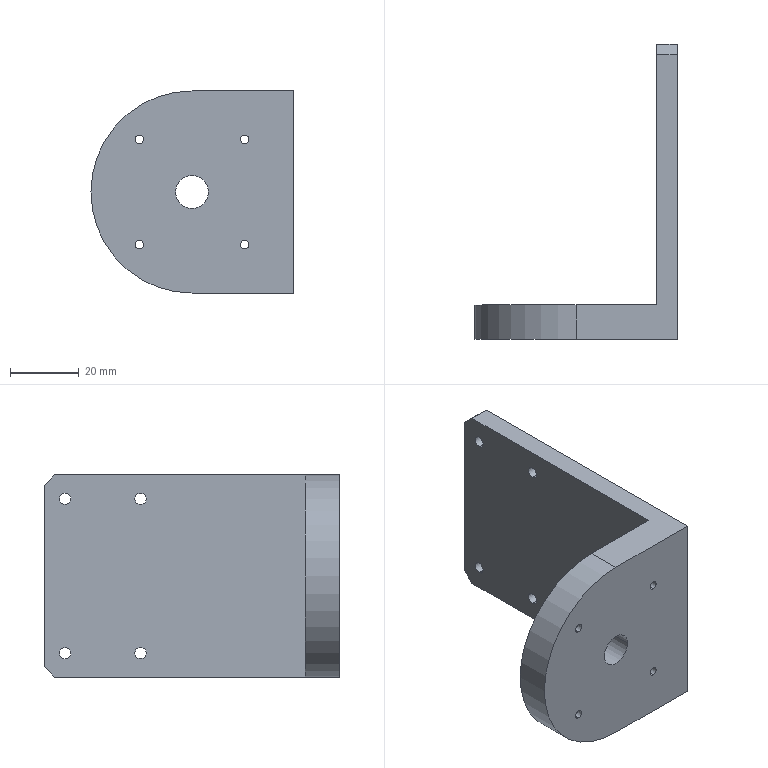Part | SolidWorks | features HoleWzd 2, ICE 2, Chamfer 1, Extrusion 1 | 1 solid | 31 faces | box 59 x 86 x 59 mm | volume 55181 mm3 | cylinder 21 | plane 10 | commonest cylinder face diameters 2.5 x8 3.3 x8 9.6 x2 33 x2 59 x1
STEP:
#1=CARTESIAN_POINT('',(15.9,80.233,-24.15));
#2=VERTEX_POINT('',#1);
#3=CARTESIAN_POINT('',(15.9,80.233,-20.85));
#4=VERTEX_POINT('',#3);
#5=CARTESIAN_POINT('',(15.9,80.233,-22.5));
#6=DIRECTION('',(-1.,0.,0.));
#7=DIRECTION('',(0.,0.,1.));
#8=AXIS2_PLACEMENT_3D('',#5,#6,#7);
#9=CIRCLE('',#8,1.65);
#10=EDGE_CURVE('',#2,#4,#9,.T.);
#11=ORIENTED_EDGE('',*,*,#10,.F.);
#12=CARTESIAN_POINT('',(10.,80.233,-24.15));
#13=VERTEX_POINT('',#12);
#14=CARTESIAN_POINT('',(10.,80.233,-24.15));
#15=DIRECTION('',(-1.,0.,0.));
#16=VECTOR('',#15,1000.);
#17=LINE('',#14,#16);
#18=EDGE_CURVE('',#2,#13,#17,.T.);
#19=ORIENTED_EDGE('',*,*,#18,.T.);
#20=CARTESIAN_POINT('',(10.,80.233,-20.85));
#21=VERTEX_POINT('',#20);
#22=CARTESIAN_POINT('',(10.,80.233,-22.5));
#23=DIRECTION('',(-1.,0.,0.));
#24=DIRECTION('',(0.,0.,1.));
#25=AXIS2_PLACEMENT_3D('',#22,#23,#24);
#26=CIRCLE('',#25,1.65);
#27=EDGE_CURVE('',#13,#21,#26,.T.);
#28=ORIENTED_EDGE('',*,*,#27,.T.);
#29=CARTESIAN_POINT('',(10.,80.233,-20.85));
#30=DIRECTION('',(-1.,0.,0.));
#31=VECTOR('',#30,1000.);
#32=LINE('',#29,#31);
#33=EDGE_CURVE('',#4,#21,#32,.T.);
#34=ORIENTED_EDGE('',*,*,#33,.F.);
#35=EDGE_LOOP('',(#11,#19,#28,#34));
#36=FACE_OUTER_BOUND('',#35,.T.);
#37=CARTESIAN_POINT('',(10.,80.233,-22.5));
#38=DIRECTION('',(-1.,0.,0.));
#39=DIRECTION('',(0.,0.,1.));
#40=AXIS2_PLACEMENT_3D('',#37,#38,#39);
#41=CYLINDRICAL_SURFACE('',#40,1.65);
#42=ADVANCED_FACE('',(#36),#41,.F.);
#43=CARTESIAN_POINT('',(15.9,58.233,-24.15));
#44=VERTEX_POINT('',#43);
#45=CARTESIAN_POINT('',(15.9,58.233,-20.85));
#46=VERTEX_POINT('',#45);
#47=CARTESIAN_POINT('',(15.9,58.233,-22.5));
#48=DIRECTION('',(-1.,0.,0.));
#49=DIRECTION('',(0.,0.,1.));
#50=AXIS2_PLACEMENT_3D('',#47,#48,#49);
#51=CIRCLE('',#50,1.65);
#52=EDGE_CURVE('',#44,#46,#51,.T.);
#53=ORIENTED_EDGE('',*,*,#52,.F.);
#54=CARTESIAN_POINT('',(10.,58.233,-24.15));
#55=VERTEX_POINT('',#54);
#56=CARTESIAN_POINT('',(10.,58.233,-24.15));
#57=DIRECTION('',(-1.,0.,0.));
#58=VECTOR('',#57,1000.);
#59=LINE('',#56,#58);
#60=EDGE_CURVE('',#44,#55,#59,.T.);
#61=ORIENTED_EDGE('',*,*,#60,.T.);
#62=CARTESIAN_POINT('',(10.,58.233,-20.85));
#63=VERTEX_POINT('',#62);
#64=CARTESIAN_POINT('',(10.,58.233,-22.5));
#65=DIRECTION('',(-1.,0.,0.));
#66=DIRECTION('',(0.,0.,1.));
#67=AXIS2_PLACEMENT_3D('',#64,#65,#66);
#68=CIRCLE('',#67,1.65);
#69=EDGE_CURVE('',#55,#63,#68,.T.);
#70=ORIENTED_EDGE('',*,*,#69,.T.);
#71=CARTESIAN_POINT('',(10.,58.233,-20.85));
#72=DIRECTION('',(-1.,0.,0.));
#73=VECTOR('',#72,1000.);
#74=LINE('',#71,#73);
#75=EDGE_CURVE('',#46,#63,#74,.T.);
#76=ORIENTED_EDGE('',*,*,#75,.F.);
#77=EDGE_LOOP('',(#53,#61,#70,#76));
#78=FACE_OUTER_BOUND('',#77,.T.);
#79=CARTESIAN_POINT('',(10.,58.233,-22.5));
#80=DIRECTION('',(-1.,0.,0.));
#81=DIRECTION('',(0.,0.,1.));
#82=AXIS2_PLACEMENT_3D('',#79,#80,#81);
#83=CYLINDRICAL_SURFACE('',#82,1.65);
#84=ADVANCED_FACE('',(#78),#83,.F.);
#85=CARTESIAN_POINT('',(15.9,58.233,20.85));
#86=VERTEX_POINT('',#85);
#87=CARTESIAN_POINT('',(15.9,58.233,24.15));
#88=VERTEX_POINT('',#87);
#89=CARTESIAN_POINT('',(15.9,58.233,22.5));
#90=DIRECTION('',(-1.,0.,0.));
#91=DIRECTION('',(0.,0.,1.));
#92=AXIS2_PLACEMENT_3D('',#89,#90,#91);
#93=CIRCLE('',#92,1.65);
#94=EDGE_CURVE('',#86,#88,#93,.T.);
#95=ORIENTED_EDGE('',*,*,#94,.F.);
#96=CARTESIAN_POINT('',(10.,58.233,20.85));
#97=VERTEX_POINT('',#96);
#98=CARTESIAN_POINT('',(10.,58.233,20.85));
#99=DIRECTION('',(-1.,0.,0.));
#100=VECTOR('',#99,1000.);
#101=LINE('',#98,#100);
#102=EDGE_CURVE('',#86,#97,#101,.T.);
#103=ORIENTED_EDGE('',*,*,#102,.T.);
#104=CARTESIAN_POINT('',(10.,58.233,24.15));
#105=VERTEX_POINT('',#104);
#106=CARTESIAN_POINT('',(10.,58.233,22.5));
#107=DIRECTION('',(-1.,0.,0.));
#108=DIRECTION('',(0.,0.,1.));
#109=AXIS2_PLACEMENT_3D('',#106,#107,#108);
#110=CIRCLE('',#109,1.65);
#111=EDGE_CURVE('',#97,#105,#110,.T.);
#112=ORIENTED_EDGE('',*,*,#111,.T.);
#113=CARTESIAN_POINT('',(10.,58.233,24.15));
#114=DIRECTION('',(-1.,0.,0.));
#115=VECTOR('',#114,1000.);
#116=LINE('',#113,#115);
#117=EDGE_CURVE('',#88,#105,#116,.T.);
#118=ORIENTED_EDGE('',*,*,#117,.F.);
#119=EDGE_LOOP('',(#95,#103,#112,#118));
#120=FACE_OUTER_BOUND('',#119,.T.);
#121=CARTESIAN_POINT('',(10.,58.233,22.5));
#122=DIRECTION('',(-1.,0.,0.));
#123=DIRECTION('',(0.,0.,1.));
#124=AXIS2_PLACEMENT_3D('',#121,#122,#123);
#125=CYLINDRICAL_SURFACE('',#124,1.65);
#126=ADVANCED_FACE('',(#120),#125,.F.);
#127=CARTESIAN_POINT('',(15.9,80.233,20.85));
#128=VERTEX_POINT('',#127);
#129=CARTESIAN_POINT('',(15.9,80.233,24.15));
#130=VERTEX_POINT('',#129);
#131=CARTESIAN_POINT('',(15.9,80.233,22.5));
#132=DIRECTION('',(-1.,0.,0.));
#133=DIRECTION('',(0.,0.,1.));
#134=AXIS2_PLACEMENT_3D('',#131,#132,#133);
#135=CIRCLE('',#134,1.65);
#136=EDGE_CURVE('',#128,#130,#135,.T.);
#137=ORIENTED_EDGE('',*,*,#136,.F.);
#138=CARTESIAN_POINT('',(10.,80.233,20.85));
#139=VERTEX_POINT('',#138);
#140=CARTESIAN_POINT('',(10.,80.233,20.85));
#141=DIRECTION('',(-1.,0.,0.));
#142=VECTOR('',#141,1000.);
#143=LINE('',#140,#142);
#144=EDGE_CURVE('',#128,#139,#143,.T.);
#145=ORIENTED_EDGE('',*,*,#144,.T.);
#146=CARTESIAN_POINT('',(10.,80.233,24.15));
#147=VERTEX_POINT('',#146);
#148=CARTESIAN_POINT('',(10.,80.233,22.5));
#149=DIRECTION('',(-1.,0.,0.));
#150=DIRECTION('',(0.,0.,1.));
#151=AXIS2_PLACEMENT_3D('',#148,#149,#150);
#152=CIRCLE('',#151,1.65);
#153=EDGE_CURVE('',#139,#147,#152,.T.);
#154=ORIENTED_EDGE('',*,*,#153,.T.);
#155=CARTESIAN_POINT('',(10.,80.233,24.15));
#156=DIRECTION('',(-1.,0.,0.));
#157=VECTOR('',#156,1000.);
#158=LINE('',#155,#157);
#159=EDGE_CURVE('',#130,#147,#158,.T.);
#160=ORIENTED_EDGE('',*,*,#159,.F.);
#161=EDGE_LOOP('',(#137,#145,#154,#160));
#162=FACE_OUTER_BOUND('',#161,.T.);
#163=CARTESIAN_POINT('',(10.,80.233,22.5));
#164=DIRECTION('',(-1.,0.,0.));
#165=DIRECTION('',(0.,0.,1.));
#166=AXIS2_PLACEMENT_3D('',#163,#164,#165);
#167=CYLINDRICAL_SURFACE('',#166,1.65);
#168=ADVANCED_FACE('',(#162),#167,.F.);
#169=CARTESIAN_POINT('',(-28.98,0.233,14.13));
#170=VERTEX_POINT('',#169);
#171=CARTESIAN_POINT('',(-28.98,0.233,16.63));
#172=VERTEX_POINT('',#171);
#173=CARTESIAN_POINT('',(-28.98,0.233,15.38));
#174=DIRECTION('',(0.,1.,0.));
#175=DIRECTION('',(0.,0.,1.));
#176=AXIS2_PLACEMENT_3D('',#173,#174,#175);
#177=CIRCLE('',#176,1.25);
#178=EDGE_CURVE('',#170,#172,#177,.T.);
#179=ORIENTED_EDGE('',*,*,#178,.F.);
#180=CARTESIAN_POINT('',(-28.98,10.233,14.13));
#181=VERTEX_POINT('',#180);
#182=CARTESIAN_POINT('',(-28.98,10.233,14.13));
#183=DIRECTION('',(0.,1.,0.));
#184=VECTOR('',#183,1000.);
#185=LINE('',#182,#184);
#186=EDGE_CURVE('',#170,#181,#185,.T.);
#187=ORIENTED_EDGE('',*,*,#186,.T.);
#188=CARTESIAN_POINT('',(-28.98,10.233,16.63));
#189=VERTEX_POINT('',#188);
#190=CARTESIAN_POINT('',(-28.98,10.233,15.38));
#191=DIRECTION('',(0.,1.,0.));
#192=DIRECTION('',(0.,0.,1.));
#193=AXIS2_PLACEMENT_3D('',#190,#191,#192);
#194=CIRCLE('',#193,1.25);
#195=EDGE_CURVE('',#181,#189,#194,.T.);
#196=ORIENTED_EDGE('',*,*,#195,.T.);
#197=CARTESIAN_POINT('',(-28.98,10.233,16.63));
#198=DIRECTION('',(0.,1.,0.));
#199=VECTOR('',#198,1000.);
#200=LINE('',#197,#199);
#201=EDGE_CURVE('',#172,#189,#200,.T.);
#202=ORIENTED_EDGE('',*,*,#201,.F.);
#203=EDGE_LOOP('',(#179,#187,#196,#202));
#204=FACE_OUTER_BOUND('',#203,.T.);
#205=CARTESIAN_POINT('',(-28.98,10.233,15.38));
#206=DIRECTION('',(0.,1.,0.));
#207=DIRECTION('',(0.,0.,1.));
#208=AXIS2_PLACEMENT_3D('',#205,#206,#207);
#209=CYLINDRICAL_SURFACE('',#208,1.25);
#210=ADVANCED_FACE('',(#204),#209,.F.);
#211=CARTESIAN_POINT('',(-28.98,0.233,-16.63));
#212=VERTEX_POINT('',#211);
#213=CARTESIAN_POINT('',(-28.98,0.233,-14.13));
#214=VERTEX_POINT('',#213);
#215=CARTESIAN_POINT('',(-28.98,0.233,-15.38));
#216=DIRECTION('',(0.,1.,0.));
#217=DIRECTION('',(0.,0.,1.));
#218=AXIS2_PLACEMENT_3D('',#215,#216,#217);
#219=CIRCLE('',#218,1.25);
#220=EDGE_CURVE('',#212,#214,#219,.T.);
#221=ORIENTED_EDGE('',*,*,#220,.F.);
#222=CARTESIAN_POINT('',(-28.98,10.233,-16.63));
#223=VERTEX_POINT('',#222);
#224=CARTESIAN_POINT('',(-28.98,10.233,-16.63));
#225=DIRECTION('',(0.,1.,0.));
#226=VECTOR('',#225,1000.);
#227=LINE('',#224,#226);
#228=EDGE_CURVE('',#212,#223,#227,.T.);
#229=ORIENTED_EDGE('',*,*,#228,.T.);
#230=CARTESIAN_POINT('',(-28.98,10.233,-14.13));
#231=VERTEX_POINT('',#230);
#232=CARTESIAN_POINT('',(-28.98,10.233,-15.38));
#233=DIRECTION('',(0.,1.,0.));
#234=DIRECTION('',(0.,0.,1.));
#235=AXIS2_PLACEMENT_3D('',#232,#233,#234);
#236=CIRCLE('',#235,1.25);
#237=EDGE_CURVE('',#223,#231,#236,.T.);
#238=ORIENTED_EDGE('',*,*,#237,.T.);
#239=CARTESIAN_POINT('',(-28.98,10.233,-14.13));
#240=DIRECTION('',(0.,1.,0.));
#241=VECTOR('',#240,1000.);
#242=LINE('',#239,#241);
#243=EDGE_CURVE('',#214,#231,#242,.T.);
#244=ORIENTED_EDGE('',*,*,#243,.F.);
#245=EDGE_LOOP('',(#221,#229,#238,#244));
#246=FACE_OUTER_BOUND('',#245,.T.);
#247=CARTESIAN_POINT('',(-28.98,10.233,-15.38));
#248=DIRECTION('',(0.,1.,0.));
#249=DIRECTION('',(0.,0.,1.));
#250=AXIS2_PLACEMENT_3D('',#247,#248,#249);
#251=CYLINDRICAL_SURFACE('',#250,1.25);
#252=ADVANCED_FACE('',(#246),#251,.F.);
#253=CARTESIAN_POINT('',(1.78,0.233,-16.63));
#254=VERTEX_POINT('',#253);
#255=CARTESIAN_POINT('',(1.78,0.233,-14.13));
#256=VERTEX_POINT('',#255);
#257=CARTESIAN_POINT('',(1.78,0.233,-15.38));
#258=DIRECTION('',(0.,1.,0.));
#259=DIRECTION('',(0.,0.,1.));
#260=AXIS2_PLACEMENT_3D('',#257,#258,#259);
#261=CIRCLE('',#260,1.25);
#262=EDGE_CURVE('',#254,#256,#261,.T.);
#263=ORIENTED_EDGE('',*,*,#262,.F.);
#264=CARTESIAN_POINT('',(1.78,10.233,-16.63));
#265=VERTEX_POINT('',#264);
#266=CARTESIAN_POINT('',(1.78,10.233,-16.63));
#267=DIRECTION('',(0.,1.,0.));
#268=VECTOR('',#267,1000.);
#269=LINE('',#266,#268);
#270=EDGE_CURVE('',#254,#265,#269,.T.);
#271=ORIENTED_EDGE('',*,*,#270,.T.);
#272=CARTESIAN_POINT('',(1.78,10.233,-14.13));
#273=VERTEX_POINT('',#272);
#274=CARTESIAN_POINT('',(1.78,10.233,-15.38));
#275=DIRECTION('',(0.,1.,0.));
#276=DIRECTION('',(0.,0.,1.));
#277=AXIS2_PLACEMENT_3D('',#274,#275,#276);
#278=CIRCLE('',#277,1.25);
#279=EDGE_CURVE('',#265,#273,#278,.T.);
#280=ORIENTED_EDGE('',*,*,#279,.T.);
#281=CARTESIAN_POINT('',(1.78,10.233,-14.13));
#282=DIRECTION('',(0.,1.,0.));
#283=VECTOR('',#282,1000.);
#284=LINE('',#281,#283);
#285=EDGE_CURVE('',#256,#273,#284,.T.);
#286=ORIENTED_EDGE('',*,*,#285,.F.);
#287=EDGE_LOOP('',(#263,#271,#280,#286));
#288=FACE_OUTER_BOUND('',#287,.T.);
#289=CARTESIAN_POINT('',(1.78,10.233,-15.38));
#290=DIRECTION('',(0.,1.,0.));
#291=DIRECTION('',(0.,0.,1.));
#292=AXIS2_PLACEMENT_3D('',#289,#290,#291);
#293=CYLINDRICAL_SURFACE('',#292,1.25);
#294=ADVANCED_FACE('',(#288),#293,.F.);
#295=CARTESIAN_POINT('',(1.78,0.233,14.13));
#296=VERTEX_POINT('',#295);
#297=CARTESIAN_POINT('',(1.78,0.233,16.63));
#298=VERTEX_POINT('',#297);
#299=CARTESIAN_POINT('',(1.78,0.233,15.38));
#300=DIRECTION('',(0.,1.,0.));
#301=DIRECTION('',(0.,0.,1.));
#302=AXIS2_PLACEMENT_3D('',#299,#300,#301);
#303=CIRCLE('',#302,1.25);
#304=EDGE_CURVE('',#296,#298,#303,.T.);
#305=ORIENTED_EDGE('',*,*,#304,.F.);
#306=CARTESIAN_POINT('',(1.78,10.233,14.13));
#307=VERTEX_POINT('',#306);
#308=CARTESIAN_POINT('',(1.78,10.233,14.13));
#309=DIRECTION('',(0.,1.,0.));
#310=VECTOR('',#309,1000.);
#311=LINE('',#308,#310);
#312=EDGE_CURVE('',#296,#307,#311,.T.);
#313=ORIENTED_EDGE('',*,*,#312,.T.);
#314=CARTESIAN_POINT('',(1.78,10.233,16.63));
#315=VERTEX_POINT('',#314);
#316=CARTESIAN_POINT('',(1.78,10.233,15.38));
#317=DIRECTION('',(0.,1.,0.));
#318=DIRECTION('',(0.,0.,1.));
#319=AXIS2_PLACEMENT_3D('',#316,#317,#318);
#320=CIRCLE('',#319,1.25);
#321=EDGE_CURVE('',#307,#315,#320,.T.);
#322=ORIENTED_EDGE('',*,*,#321,.T.);
#323=CARTESIAN_POINT('',(1.78,10.233,16.63));
#324=DIRECTION('',(0.,1.,0.));
#325=VECTOR('',#324,1000.);
#326=LINE('',#323,#325);
#327=EDGE_CURVE('',#298,#315,#326,.T.);
#328=ORIENTED_EDGE('',*,*,#327,.F.);
#329=EDGE_LOOP('',(#305,#313,#322,#328));
#330=FACE_OUTER_BOUND('',#329,.T.);
#331=CARTESIAN_POINT('',(1.78,10.233,15.38));
#332=DIRECTION('',(0.,1.,0.));
#333=DIRECTION('',(0.,0.,1.));
#334=AXIS2_PLACEMENT_3D('',#331,#332,#333);
#335=CYLINDRICAL_SURFACE('',#334,1.25);
#336=ADVANCED_FACE('',(#330),#335,.F.);
#337=CARTESIAN_POINT('',(2.9,8.733,0.));
#338=VERTEX_POINT('',#337);
#339=CARTESIAN_POINT('',(-30.1,8.733,0.));
#340=VERTEX_POINT('',#339);
#341=CARTESIAN_POINT('',(-13.6,8.733,0.));
#342=DIRECTION('',(0.,1.,0.));
#343=DIRECTION('',(-1.,0.,0.));
#344=AXIS2_PLACEMENT_3D('',#341,#342,#343);
#345=CIRCLE('',#344,16.5);
#346=EDGE_CURVE('',#338,#340,#345,.T.);
#347=ORIENTED_EDGE('',*,*,#346,.F.);
#348=CARTESIAN_POINT('',(2.9,10.233,0.));
#349=VERTEX_POINT('',#348);
#350=CARTESIAN_POINT('',(2.9,8.733,0.));
#351=DIRECTION('',(0.,1.,0.));
#352=VECTOR('',#351,1000.);
#353=LINE('',#350,#352);
#354=EDGE_CURVE('',#338,#349,#353,.T.);
#355=ORIENTED_EDGE('',*,*,#354,.T.);
#356=CARTESIAN_POINT('',(-30.1,10.233,0.));
#357=VERTEX_POINT('',#356);
#358=CARTESIAN_POINT('',(-13.6,10.233,0.));
#359=DIRECTION('',(0.,1.,0.));
#360=DIRECTION('',(-1.,0.,0.));
#361=AXIS2_PLACEMENT_3D('',#358,#359,#360);
#362=CIRCLE('',#361,16.5);
#363=EDGE_CURVE('',#349,#357,#362,.T.);
#364=ORIENTED_EDGE('',*,*,#363,.T.);
#365=CARTESIAN_POINT('',(-30.1,8.733,0.));
#366=DIRECTION('',(0.,1.,0.));
#367=VECTOR('',#366,1000.);
#368=LINE('',#365,#367);
#369=EDGE_CURVE('',#340,#357,#368,.T.);
#370=ORIENTED_EDGE('',*,*,#369,.F.);
#371=EDGE_LOOP('',(#347,#355,#364,#370));
#372=FACE_OUTER_BOUND('',#371,.T.);
#373=CARTESIAN_POINT('',(-13.6,8.733,0.));
#374=DIRECTION('',(0.,1.,0.));
#375=DIRECTION('',(-1.,0.,0.));
#376=AXIS2_PLACEMENT_3D('',#373,#374,#375);
#377=CYLINDRICAL_SURFACE('',#376,16.5);
#378=ADVANCED_FACE('',(#372),#377,.F.);
#379=CARTESIAN_POINT('',(-18.4,8.733,0.));
#380=VERTEX_POINT('',#379);
#381=CARTESIAN_POINT('',(-8.8,8.733,0.));
#382=VERTEX_POINT('',#381);
#383=CARTESIAN_POINT('',(-13.6,8.733,0.));
#384=DIRECTION('',(0.,-1.,0.));
#385=DIRECTION('',(-1.,0.,0.));
#386=AXIS2_PLACEMENT_3D('',#383,#384,#385);
#387=CIRCLE('',#386,4.8);
#388=EDGE_CURVE('',#380,#382,#387,.T.);
#389=ORIENTED_EDGE('',*,*,#388,.F.);
#390=CARTESIAN_POINT('',(-18.4,0.233,0.));
#391=VERTEX_POINT('',#390);
#392=CARTESIAN_POINT('',(-18.4,10.233,0.));
#393=DIRECTION('',(0.,-1.,0.));
#394=VECTOR('',#393,1000.);
#395=LINE('',#392,#394);
#396=EDGE_CURVE('',#380,#391,#395,.T.);
#397=ORIENTED_EDGE('',*,*,#396,.T.);
#398=CARTESIAN_POINT('',(-8.8,0.233,0.));
#399=VERTEX_POINT('',#398);
#400=CARTESIAN_POINT('',(-13.6,0.233,0.));
#401=DIRECTION('',(0.,-1.,0.));
#402=DIRECTION('',(1.,0.,0.));
#403=AXIS2_PLACEMENT_3D('',#400,#401,#402);
#404=CIRCLE('',#403,4.8);
#405=EDGE_CURVE('',#391,#399,#404,.T.);
#406=ORIENTED_EDGE('',*,*,#405,.T.);
#407=CARTESIAN_POINT('',(-8.8,10.233,0.));
#408=DIRECTION('',(0.,-1.,0.));
#409=VECTOR('',#408,1000.);
#410=LINE('',#407,#409);
#411=EDGE_CURVE('',#382,#399,#410,.T.);
#412=ORIENTED_EDGE('',*,*,#411,.F.);
#413=EDGE_LOOP('',(#389,#397,#406,#412));
#414=FACE_OUTER_BOUND('',#413,.T.);
#415=CARTESIAN_POINT('',(-13.6,10.233,0.));
#416=DIRECTION('',(0.,-1.,0.));
#417=DIRECTION('',(1.,0.,0.));
#418=AXIS2_PLACEMENT_3D('',#415,#416,#417);
#419=CYLINDRICAL_SURFACE('',#418,4.8);
#420=ADVANCED_FACE('',(#414),#419,.F.);
#421=ORIENTED_EDGE('',*,*,#396,.F.);
#422=CARTESIAN_POINT('',(-13.6,8.733,0.));
#423=DIRECTION('',(0.,-1.,0.));
#424=DIRECTION('',(-1.,0.,0.));
#425=AXIS2_PLACEMENT_3D('',#422,#423,#424);
#426=CIRCLE('',#425,4.8);
#427=EDGE_CURVE('',#382,#380,#426,.T.);
#428=ORIENTED_EDGE('',*,*,#427,.F.);
#429=ORIENTED_EDGE('',*,*,#411,.T.);
#430=CARTESIAN_POINT('',(-13.6,0.233,0.));
#431=DIRECTION('',(0.,-1.,0.));
#432=DIRECTION('',(1.,0.,0.));
#433=AXIS2_PLACEMENT_3D('',#430,#431,#432);
#434=CIRCLE('',#433,4.8);
#435=EDGE_CURVE('',#399,#391,#434,.T.);
#436=ORIENTED_EDGE('',*,*,#435,.T.);
#437=EDGE_LOOP('',(#421,#428,#429,#436));
#438=FACE_OUTER_BOUND('',#437,.T.);
#439=CARTESIAN_POINT('',(-13.6,10.233,0.));
#440=DIRECTION('',(0.,-1.,0.));
#441=DIRECTION('',(1.,0.,0.));
#442=AXIS2_PLACEMENT_3D('',#439,#440,#441);
#443=CYLINDRICAL_SURFACE('',#442,4.8);
#444=ADVANCED_FACE('',(#438),#443,.F.);
#445=CARTESIAN_POINT('',(-28.98,10.233,15.38));
#446=DIRECTION('',(0.,1.,0.));
#447=DIRECTION('',(0.,0.,1.));
#448=AXIS2_PLACEMENT_3D('',#445,#446,#447);
#449=CIRCLE('',#448,1.25);
#450=EDGE_CURVE('',#189,#181,#449,.T.);
#451=ORIENTED_EDGE('',*,*,#450,.F.);
#452=ORIENTED_EDGE('',*,*,#195,.F.);
#453=EDGE_LOOP('',(#451,#452));
#454=FACE_BOUND('',#453,.T.);
#455=CARTESIAN_POINT('',(-28.98,10.233,-15.38));
#456=DIRECTION('',(0.,1.,0.));
#457=DIRECTION('',(0.,0.,1.));
#458=AXIS2_PLACEMENT_3D('',#455,#456,#457);
#459=CIRCLE('',#458,1.25);
#460=EDGE_CURVE('',#231,#223,#459,.T.);
#461=ORIENTED_EDGE('',*,*,#460,.F.);
#462=ORIENTED_EDGE('',*,*,#237,.F.);
#463=EDGE_LOOP('',(#461,#462));
#464=FACE_BOUND('',#463,.T.);
#465=CARTESIAN_POINT('',(1.78,10.233,-15.38));
#466=DIRECTION('',(0.,1.,0.));
#467=DIRECTION('',(0.,0.,1.));
#468=AXIS2_PLACEMENT_3D('',#465,#466,#467);
#469=CIRCLE('',#468,1.25);
#470=EDGE_CURVE('',#273,#265,#469,.T.);
#471=ORIENTED_EDGE('',*,*,#470,.F.);
#472=ORIENTED_EDGE('',*,*,#279,.F.);
#473=EDGE_LOOP('',(#471,#472));
#474=FACE_BOUND('',#473,.T.);
#475=CARTESIAN_POINT('',(1.78,10.233,15.38));
#476=DIRECTION('',(0.,1.,0.));
#477=DIRECTION('',(0.,0.,1.));
#478=AXIS2_PLACEMENT_3D('',#475,#476,#477);
#479=CIRCLE('',#478,1.25);
#480=EDGE_CURVE('',#315,#307,#479,.T.);
#481=ORIENTED_EDGE('',*,*,#480,.F.);
#482=ORIENTED_EDGE('',*,*,#321,.F.);
#483=EDGE_LOOP('',(#481,#482));
#484=FACE_BOUND('',#483,.T.);
#485=CARTESIAN_POINT('',(-13.6,10.233,0.));
#486=DIRECTION('',(0.,1.,0.));
#487=DIRECTION('',(-1.,0.,0.));
#488=AXIS2_PLACEMENT_3D('',#485,#486,#487);
#489=CIRCLE('',#488,16.5);
#490=EDGE_CURVE('',#357,#349,#489,.T.);
#491=ORIENTED_EDGE('',*,*,#490,.F.);
#492=ORIENTED_EDGE('',*,*,#363,.F.);
#493=EDGE_LOOP('',(#491,#492));
#494=FACE_BOUND('',#493,.T.);
#495=CARTESIAN_POINT('',(10.,10.233,-29.5));
#496=VERTEX_POINT('',#495);
#497=CARTESIAN_POINT('',(-13.6,10.233,-29.5));
#498=VERTEX_POINT('',#497);
#499=CARTESIAN_POINT('',(10.,10.233,-29.5));
#500=DIRECTION('',(-1.,0.,0.));
#501=VECTOR('',#500,1000.);
#502=LINE('',#499,#501);
#503=EDGE_CURVE('',#496,#498,#502,.T.);
#504=ORIENTED_EDGE('',*,*,#503,.T.);
#505=CARTESIAN_POINT('',(-13.6,10.233,29.5));
#506=VERTEX_POINT('',#505);
#507=CARTESIAN_POINT('',(-13.6,10.233,0.));
#508=DIRECTION('',(0.,-1.,0.));
#509=DIRECTION('',(1.,0.,0.));
#510=AXIS2_PLACEMENT_3D('',#507,#508,#509);
#511=CIRCLE('',#510,29.5);
#512=EDGE_CURVE('',#506,#498,#511,.T.);
#513=ORIENTED_EDGE('',*,*,#512,.F.);
#514=CARTESIAN_POINT('',(10.,10.233,29.5));
#515=VERTEX_POINT('',#514);
#516=CARTESIAN_POINT('',(10.,10.233,29.5));
#517=DIRECTION('',(-1.,0.,0.));
#518=VECTOR('',#517,1000.);
#519=LINE('',#516,#518);
#520=EDGE_CURVE('',#515,#506,#519,.T.);
#521=ORIENTED_EDGE('',*,*,#520,.F.);
#522=CARTESIAN_POINT('',(10.,10.233,29.5));
#523=DIRECTION('',(0.,0.,-1.));
#524=VECTOR('',#523,1000.);
#525=LINE('',#522,#524);
#526=EDGE_CURVE('',#515,#496,#525,.T.);
#527=ORIENTED_EDGE('',*,*,#526,.T.);
#528=EDGE_LOOP('',(#504,#513,#521,#527));
#529=FACE_OUTER_BOUND('',#528,.T.);
#530=CARTESIAN_POINT('',(10.,10.233,29.5));
#531=DIRECTION('',(0.,-1.,0.));
#532=DIRECTION('',(1.,0.,0.));
#533=AXIS2_PLACEMENT_3D('',#530,#531,#532);
#534=PLANE('',#533);
#535=ADVANCED_FACE('',(#454,#464,#474,#484,#494,#529),#534,.F.);
#536=CARTESIAN_POINT('',(-28.98,0.233,15.38));
#537=DIRECTION('',(0.,1.,0.));
#538=DIRECTION('',(0.,0.,1.));
#539=AXIS2_PLACEMENT_3D('',#536,#537,#538);
#540=CIRCLE('',#539,1.25);
#541=EDGE_CURVE('',#172,#170,#540,.T.);
#542=ORIENTED_EDGE('',*,*,#541,.T.);
#543=ORIENTED_EDGE('',*,*,#178,.T.);
#544=EDGE_LOOP('',(#542,#543));
#545=FACE_BOUND('',#544,.T.);
#546=CARTESIAN_POINT('',(-28.98,0.233,-15.38));
#547=DIRECTION('',(0.,1.,0.));
#548=DIRECTION('',(0.,0.,1.));
#549=AXIS2_PLACEMENT_3D('',#546,#547,#548);
#550=CIRCLE('',#549,1.25);
#551=EDGE_CURVE('',#214,#212,#550,.T.);
#552=ORIENTED_EDGE('',*,*,#551,.T.);
#553=ORIENTED_EDGE('',*,*,#220,.T.);
#554=EDGE_LOOP('',(#552,#553));
#555=FACE_BOUND('',#554,.T.);
#556=CARTESIAN_POINT('',(1.78,0.233,-15.38));
#557=DIRECTION('',(0.,1.,0.));
#558=DIRECTION('',(0.,0.,1.));
#559=AXIS2_PLACEMENT_3D('',#556,#557,#558);
#560=CIRCLE('',#559,1.25);
#561=EDGE_CURVE('',#256,#254,#560,.T.);
#562=ORIENTED_EDGE('',*,*,#561,.T.);
#563=ORIENTED_EDGE('',*,*,#262,.T.);
#564=EDGE_LOOP('',(#562,#563));
#565=FACE_BOUND('',#564,.T.);
#566=CARTESIAN_POINT('',(1.78,0.233,15.38));
#567=DIRECTION('',(0.,1.,0.));
#568=DIRECTION('',(0.,0.,1.));
#569=AXIS2_PLACEMENT_3D('',#566,#567,#568);
#570=CIRCLE('',#569,1.25);
#571=EDGE_CURVE('',#298,#296,#570,.T.);
#572=ORIENTED_EDGE('',*,*,#571,.T.);
#573=ORIENTED_EDGE('',*,*,#304,.T.);
#574=EDGE_LOOP('',(#572,#573));
#575=FACE_BOUND('',#574,.T.);
#576=ORIENTED_EDGE('',*,*,#435,.F.);
#577=ORIENTED_EDGE('',*,*,#405,.F.);
#578=EDGE_LOOP('',(#576,#577));
#579=FACE_BOUND('',#578,.T.);
#580=CARTESIAN_POINT('',(-13.6,0.233,29.5));
#581=VERTEX_POINT('',#580);
#582=CARTESIAN_POINT('',(-13.6,0.233,-29.5));
#583=VERTEX_POINT('',#582);
#584=CARTESIAN_POINT('',(-13.6,0.233,0.));
#585=DIRECTION('',(0.,-1.,0.));
#586=DIRECTION('',(1.,0.,0.));
#587=AXIS2_PLACEMENT_3D('',#584,#585,#586);
#588=CIRCLE('',#587,29.5);
#589=EDGE_CURVE('',#581,#583,#588,.T.);
#590=ORIENTED_EDGE('',*,*,#589,.T.);
#591=CARTESIAN_POINT('',(15.9,0.233,-29.5));
#592=VERTEX_POINT('',#591);
#593=CARTESIAN_POINT('',(15.9,0.233,-29.5));
#594=DIRECTION('',(1.,0.,0.));
#595=VECTOR('',#594,1000.);
#596=LINE('',#593,#595);
#597=EDGE_CURVE('',#583,#592,#596,.T.);
#598=ORIENTED_EDGE('',*,*,#597,.T.);
#599=CARTESIAN_POINT('',(15.9,0.233,29.5));
#600=VERTEX_POINT('',#599);
#601=CARTESIAN_POINT('',(15.9,0.233,29.5));
#602=DIRECTION('',(0.,0.,-1.));
#603=VECTOR('',#602,1000.);
#604=LINE('',#601,#603);
#605=EDGE_CURVE('',#600,#592,#604,.T.);
#606=ORIENTED_EDGE('',*,*,#605,.F.);
#607=CARTESIAN_POINT('',(15.9,0.233,29.5));
#608=DIRECTION('',(1.,0.,0.));
#609=VECTOR('',#608,1000.);
#610=LINE('',#607,#609);
#611=EDGE_CURVE('',#581,#600,#610,.T.);
#612=ORIENTED_EDGE('',*,*,#611,.F.);
#613=EDGE_LOOP('',(#590,#598,#606,#612));
#614=FACE_OUTER_BOUND('',#613,.T.);
#615=CARTESIAN_POINT('',(15.9,0.233,29.5));
#616=DIRECTION('',(0.,1.,0.));
#617=DIRECTION('',(-1.,0.,0.));
#618=AXIS2_PLACEMENT_3D('',#615,#616,#617);
#619=PLANE('',#618);
#620=ADVANCED_FACE('',(#545,#555,#565,#575,#579,#614),#619,.F.);
#621=CARTESIAN_POINT('',(10.,83.233,-29.5));
#622=VERTEX_POINT('',#621);
#623=CARTESIAN_POINT('',(10.,86.233,-29.5));
#624=DIRECTION('',(0.,-1.,0.));
#625=VECTOR('',#624,1000.);
#626=LINE('',#623,#625);
#627=EDGE_CURVE('',#622,#496,#626,.T.);
#628=ORIENTED_EDGE('',*,*,#627,.F.);
#629=CARTESIAN_POINT('',(15.9,83.233,-29.5));
#630=VERTEX_POINT('',#629);
#631=CARTESIAN_POINT('',(0.,83.233,-29.5));
#632=DIRECTION('',(1.,0.,0.));
#633=VECTOR('',#632,1000.);
#634=LINE('',#631,#633);
#635=EDGE_CURVE('',#622,#630,#634,.T.);
#636=ORIENTED_EDGE('',*,*,#635,.T.);
#637=CARTESIAN_POINT('',(15.9,0.233,-29.5));
#638=DIRECTION('',(0.,1.,0.));
#639=VECTOR('',#638,1000.);
#640=LINE('',#637,#639);
#641=EDGE_CURVE('',#592,#630,#640,.T.);
#642=ORIENTED_EDGE('',*,*,#641,.F.);
#643=ORIENTED_EDGE('',*,*,#597,.F.);
#644=CARTESIAN_POINT('',(-13.6,10.233,-29.5));
#645=DIRECTION('',(0.,-1.,0.));
#646=VECTOR('',#645,1000.);
#647=LINE('',#644,#646);
#648=EDGE_CURVE('',#498,#583,#647,.T.);
#649=ORIENTED_EDGE('',*,*,#648,.F.);
#650=ORIENTED_EDGE('',*,*,#503,.F.);
#651=EDGE_LOOP('',(#628,#636,#642,#643,#649,#650));
#652=FACE_OUTER_BOUND('',#651,.T.);
#653=CARTESIAN_POINT('',(0.,0.,-29.5));
#654=DIRECTION('',(0.,0.,1.));
#655=DIRECTION('',(1.,0.,0.));
#656=AXIS2_PLACEMENT_3D('',#653,#654,#655);
#657=PLANE('',#656);
#658=ADVANCED_FACE('',(#652),#657,.F.);
#659=CARTESIAN_POINT('',(15.9,83.233,29.5));
#660=VERTEX_POINT('',#659);
#661=CARTESIAN_POINT('',(15.9,0.233,29.5));
#662=DIRECTION('',(0.,1.,0.));
#663=VECTOR('',#662,1000.);
#664=LINE('',#661,#663);
#665=EDGE_CURVE('',#600,#660,#664,.T.);
#666=ORIENTED_EDGE('',*,*,#665,.T.);
#667=CARTESIAN_POINT('',(10.,83.233,29.5));
#668=VERTEX_POINT('',#667);
#669=CARTESIAN_POINT('',(10.,83.233,29.5));
#670=DIRECTION('',(-1.,0.,0.));
#671=VECTOR('',#670,1000.);
#672=LINE('',#669,#671);
#673=EDGE_CURVE('',#660,#668,#672,.T.);
#674=ORIENTED_EDGE('',*,*,#673,.T.);
#675=CARTESIAN_POINT('',(10.,86.233,29.5));
#676=DIRECTION('',(0.,-1.,0.));
#677=VECTOR('',#676,1000.);
#678=LINE('',#675,#677);
#679=EDGE_CURVE('',#668,#515,#678,.T.);
#680=ORIENTED_EDGE('',*,*,#679,.T.);
#681=ORIENTED_EDGE('',*,*,#520,.T.);
#682=CARTESIAN_POINT('',(-13.6,10.233,29.5));
#683=DIRECTION('',(0.,-1.,0.));
#684=VECTOR('',#683,1000.);
#685=LINE('',#682,#684);
#686=EDGE_CURVE('',#506,#581,#685,.T.);
#687=ORIENTED_EDGE('',*,*,#686,.T.);
#688=ORIENTED_EDGE('',*,*,#611,.T.);
#689=EDGE_LOOP('',(#666,#674,#680,#681,#687,#688));
#690=FACE_OUTER_BOUND('',#689,.T.);
#691=CARTESIAN_POINT('',(0.,0.,29.5));
#692=DIRECTION('',(0.,0.,1.));
#693=DIRECTION('',(1.,0.,0.));
#694=AXIS2_PLACEMENT_3D('',#691,#692,#693);
#695=PLANE('',#694);
#696=ADVANCED_FACE('',(#690),#695,.T.);
#697=CARTESIAN_POINT('',(15.9,80.233,-22.5));
#698=DIRECTION('',(-1.,0.,0.));
#699=DIRECTION('',(0.,0.,1.));
#700=AXIS2_PLACEMENT_3D('',#697,#698,#699);
#701=CIRCLE('',#700,1.65);
#702=EDGE_CURVE('',#4,#2,#701,.T.);
#703=ORIENTED_EDGE('',*,*,#702,.T.);
#704=ORIENTED_EDGE('',*,*,#10,.T.);
#705=EDGE_LOOP('',(#703,#704));
#706=FACE_BOUND('',#705,.T.);
#707=CARTESIAN_POINT('',(15.9,58.233,-22.5));
#708=DIRECTION('',(-1.,0.,0.));
#709=DIRECTION('',(0.,0.,1.));
#710=AXIS2_PLACEMENT_3D('',#707,#708,#709);
#711=CIRCLE('',#710,1.65);
#712=EDGE_CURVE('',#46,#44,#711,.T.);
#713=ORIENTED_EDGE('',*,*,#712,.T.);
#714=ORIENTED_EDGE('',*,*,#52,.T.);
#715=EDGE_LOOP('',(#713,#714));
#716=FACE_BOUND('',#715,.T.);
#717=CARTESIAN_POINT('',(15.9,58.233,22.5));
#718=DIRECTION('',(-1.,0.,0.));
#719=DIRECTION('',(0.,0.,1.));
#720=AXIS2_PLACEMENT_3D('',#717,#718,#719);
#721=CIRCLE('',#720,1.65);
#722=EDGE_CURVE('',#88,#86,#721,.T.);
#723=ORIENTED_EDGE('',*,*,#722,.T.);
#724=ORIENTED_EDGE('',*,*,#94,.T.);
#725=EDGE_LOOP('',(#723,#724));
#726=FACE_BOUND('',#725,.T.);
#727=CARTESIAN_POINT('',(15.9,80.233,22.5));
#728=DIRECTION('',(-1.,0.,0.));
#729=DIRECTION('',(0.,0.,1.));
#730=AXIS2_PLACEMENT_3D('',#727,#728,#729);
#731=CIRCLE('',#730,1.65);
#732=EDGE_CURVE('',#130,#128,#731,.T.);
#733=ORIENTED_EDGE('',*,*,#732,.T.);
#734=ORIENTED_EDGE('',*,*,#136,.T.);
#735=EDGE_LOOP('',(#733,#734));
#736=FACE_BOUND('',#735,.T.);
#737=CARTESIAN_POINT('',(15.9,86.233,26.5));
#738=VERTEX_POINT('',#737);
#739=CARTESIAN_POINT('',(15.9,86.233,-26.5));
#740=VERTEX_POINT('',#739);
#741=CARTESIAN_POINT('',(15.9,86.233,29.5));
#742=DIRECTION('',(0.,0.,-1.));
#743=VECTOR('',#742,1000.);
#744=LINE('',#741,#743);
#745=EDGE_CURVE('',#738,#740,#744,.T.);
#746=ORIENTED_EDGE('',*,*,#745,.F.);
#747=CARTESIAN_POINT('',(15.9,83.233,29.5));
#748=DIRECTION('',(0.,-0.7071,0.7071));
#749=VECTOR('',#748,1000.);
#750=LINE('',#747,#749);
#751=EDGE_CURVE('',#738,#660,#750,.T.);
#752=ORIENTED_EDGE('',*,*,#751,.T.);
#753=ORIENTED_EDGE('',*,*,#665,.F.);
#754=ORIENTED_EDGE('',*,*,#605,.T.);
#755=ORIENTED_EDGE('',*,*,#641,.T.);
#756=CARTESIAN_POINT('',(15.9,86.233,-26.5));
#757=DIRECTION('',(0.,0.7071,0.7071));
#758=VECTOR('',#757,1000.);
#759=LINE('',#756,#758);
#760=EDGE_CURVE('',#630,#740,#759,.T.);
#761=ORIENTED_EDGE('',*,*,#760,.T.);
#762=EDGE_LOOP('',(#746,#752,#753,#754,#755,#761));
#763=FACE_OUTER_BOUND('',#762,.T.);
#764=CARTESIAN_POINT('',(15.9,0.233,29.5));
#765=DIRECTION('',(-1.,0.,0.));
#766=DIRECTION('',(0.,0.,1.));
#767=AXIS2_PLACEMENT_3D('',#764,#765,#766);
#768=PLANE('',#767);
#769=ADVANCED_FACE('',(#706,#716,#726,#736,#763),#768,.F.);
#770=CARTESIAN_POINT('',(10.,86.233,26.5));
#771=VERTEX_POINT('',#770);
#772=CARTESIAN_POINT('',(10.,86.233,-26.5));
#773=VERTEX_POINT('',#772);
#774=CARTESIAN_POINT('',(10.,86.233,29.5));
#775=DIRECTION('',(0.,0.,-1.));
#776=VECTOR('',#775,1000.);
#777=LINE('',#774,#776);
#778=EDGE_CURVE('',#771,#773,#777,.T.);
#779=ORIENTED_EDGE('',*,*,#778,.F.);
#780=CARTESIAN_POINT('',(15.9,86.233,26.5));
#781=DIRECTION('',(1.,0.,0.));
#782=VECTOR('',#781,1000.);
#783=LINE('',#780,#782);
#784=EDGE_CURVE('',#771,#738,#783,.T.);
#785=ORIENTED_EDGE('',*,*,#784,.T.);
#786=ORIENTED_EDGE('',*,*,#745,.T.);
#787=CARTESIAN_POINT('',(15.9,86.233,-26.5));
#788=DIRECTION('',(-1.,0.,0.));
#789=VECTOR('',#788,1000.);
#790=LINE('',#787,#789);
#791=EDGE_CURVE('',#740,#773,#790,.T.);
#792=ORIENTED_EDGE('',*,*,#791,.T.);
#793=EDGE_LOOP('',(#779,#785,#786,#792));
#794=FACE_OUTER_BOUND('',#793,.T.);
#795=CARTESIAN_POINT('',(15.9,86.233,29.5));
#796=DIRECTION('',(0.,-1.,0.));
#797=DIRECTION('',(0.,0.,-1.));
#798=AXIS2_PLACEMENT_3D('',#795,#796,#797);
#799=PLANE('',#798);
#800=ADVANCED_FACE('',(#794),#799,.F.);
#801=CARTESIAN_POINT('',(10.,80.233,-22.5));
#802=DIRECTION('',(-1.,0.,0.));
#803=DIRECTION('',(0.,0.,1.));
#804=AXIS2_PLACEMENT_3D('',#801,#802,#803);
#805=CIRCLE('',#804,1.65);
#806=EDGE_CURVE('',#21,#13,#805,.T.);
#807=ORIENTED_EDGE('',*,*,#806,.F.);
#808=ORIENTED_EDGE('',*,*,#27,.F.);
#809=EDGE_LOOP('',(#807,#808));
#810=FACE_BOUND('',#809,.T.);
#811=CARTESIAN_POINT('',(10.,58.233,-22.5));
#812=DIRECTION('',(-1.,0.,0.));
#813=DIRECTION('',(0.,0.,1.));
#814=AXIS2_PLACEMENT_3D('',#811,#812,#813);
#815=CIRCLE('',#814,1.65);
#816=EDGE_CURVE('',#63,#55,#815,.T.);
#817=ORIENTED_EDGE('',*,*,#816,.F.);
#818=ORIENTED_EDGE('',*,*,#69,.F.);
#819=EDGE_LOOP('',(#817,#818));
#820=FACE_BOUND('',#819,.T.);
#821=CARTESIAN_POINT('',(10.,58.233,22.5));
#822=DIRECTION('',(-1.,0.,0.));
#823=DIRECTION('',(0.,0.,1.));
#824=AXIS2_PLACEMENT_3D('',#821,#822,#823);
#825=CIRCLE('',#824,1.65);
#826=EDGE_CURVE('',#105,#97,#825,.T.);
#827=ORIENTED_EDGE('',*,*,#826,.F.);
#828=ORIENTED_EDGE('',*,*,#111,.F.);
#829=EDGE_LOOP('',(#827,#828));
#830=FACE_BOUND('',#829,.T.);
#831=CARTESIAN_POINT('',(10.,80.233,22.5));
#832=DIRECTION('',(-1.,0.,0.));
#833=DIRECTION('',(0.,0.,1.));
#834=AXIS2_PLACEMENT_3D('',#831,#832,#833);
#835=CIRCLE('',#834,1.65);
#836=EDGE_CURVE('',#147,#139,#835,.T.);
#837=ORIENTED_EDGE('',*,*,#836,.F.);
#838=ORIENTED_EDGE('',*,*,#153,.F.);
#839=EDGE_LOOP('',(#837,#838));
#840=FACE_BOUND('',#839,.T.);
#841=ORIENTED_EDGE('',*,*,#679,.F.);
#842=CARTESIAN_POINT('',(10.,83.233,29.5));
#843=DIRECTION('',(0.,0.7071,-0.7071));
#844=VECTOR('',#843,1000.);
#845=LINE('',#842,#844);
#846=EDGE_CURVE('',#668,#771,#845,.T.);
#847=ORIENTED_EDGE('',*,*,#846,.T.);
#848=ORIENTED_EDGE('',*,*,#778,.T.);
#849=CARTESIAN_POINT('',(10.,86.233,-26.5));
#850=DIRECTION('',(0.,-0.7071,-0.7071));
#851=VECTOR('',#850,1000.);
#852=LINE('',#849,#851);
#853=EDGE_CURVE('',#773,#622,#852,.T.);
#854=ORIENTED_EDGE('',*,*,#853,.T.);
#855=ORIENTED_EDGE('',*,*,#627,.T.);
#856=ORIENTED_EDGE('',*,*,#526,.F.);
#857=EDGE_LOOP('',(#841,#847,#848,#854,#855,#856));
#858=FACE_OUTER_BOUND('',#857,.T.);
#859=CARTESIAN_POINT('',(10.,86.233,29.5));
#860=DIRECTION('',(1.,0.,0.));
#861=DIRECTION('',(0.,0.,-1.));
#862=AXIS2_PLACEMENT_3D('',#859,#860,#861);
#863=PLANE('',#862);
#864=ADVANCED_FACE('',(#810,#820,#830,#840,#858),#863,.F.);
#865=ORIENTED_EDGE('',*,*,#589,.F.);
#866=ORIENTED_EDGE('',*,*,#686,.F.);
#867=ORIENTED_EDGE('',*,*,#512,.T.);
#868=ORIENTED_EDGE('',*,*,#648,.T.);
#869=EDGE_LOOP('',(#865,#866,#867,#868));
#870=FACE_OUTER_BOUND('',#869,.T.);
#871=CARTESIAN_POINT('',(-13.6,10.233,0.));
#872=DIRECTION('',(0.,-1.,0.));
#873=DIRECTION('',(1.,0.,0.));
#874=AXIS2_PLACEMENT_3D('',#871,#872,#873);
#875=CYLINDRICAL_SURFACE('',#874,29.5);
#876=ADVANCED_FACE('',(#870),#875,.T.);
#877=CARTESIAN_POINT('',(-13.6,8.733,0.));
#878=DIRECTION('',(0.,1.,0.));
#879=DIRECTION('',(-1.,0.,0.));
#880=AXIS2_PLACEMENT_3D('',#877,#878,#879);
#881=CIRCLE('',#880,16.5);
#882=EDGE_CURVE('',#340,#338,#881,.T.);
#883=ORIENTED_EDGE('',*,*,#882,.T.);
#884=ORIENTED_EDGE('',*,*,#346,.T.);
#885=EDGE_LOOP('',(#883,#884));
#886=FACE_OUTER_BOUND('',#885,.T.);
#887=ORIENTED_EDGE('',*,*,#427,.T.);
#888=ORIENTED_EDGE('',*,*,#388,.T.);
#889=EDGE_LOOP('',(#887,#888));
#890=FACE_BOUND('',#889,.T.);
#891=CARTESIAN_POINT('',(-13.6,8.733,0.));
#892=DIRECTION('',(0.,1.,0.));
#893=DIRECTION('',(-1.,0.,0.));
#894=AXIS2_PLACEMENT_3D('',#891,#892,#893);
#895=PLANE('',#894);
#896=ADVANCED_FACE('',(#886,#890),#895,.T.);
#897=ORIENTED_EDGE('',*,*,#354,.F.);
#898=ORIENTED_EDGE('',*,*,#882,.F.);
#899=ORIENTED_EDGE('',*,*,#369,.T.);
#900=ORIENTED_EDGE('',*,*,#490,.T.);
#901=EDGE_LOOP('',(#897,#898,#899,#900));
#902=FACE_OUTER_BOUND('',#901,.T.);
#903=CARTESIAN_POINT('',(-13.6,8.733,0.));
#904=DIRECTION('',(0.,1.,0.));
#905=DIRECTION('',(-1.,0.,0.));
#906=AXIS2_PLACEMENT_3D('',#903,#904,#905);
#907=CYLINDRICAL_SURFACE('',#906,16.5);
#908=ADVANCED_FACE('',(#902),#907,.F.);
#909=ORIENTED_EDGE('',*,*,#312,.F.);
#910=ORIENTED_EDGE('',*,*,#571,.F.);
#911=ORIENTED_EDGE('',*,*,#327,.T.);
#912=ORIENTED_EDGE('',*,*,#480,.T.);
#913=EDGE_LOOP('',(#909,#910,#911,#912));
#914=FACE_OUTER_BOUND('',#913,.T.);
#915=CARTESIAN_POINT('',(1.78,10.233,15.38));
#916=DIRECTION('',(0.,1.,0.));
#917=DIRECTION('',(0.,0.,1.));
#918=AXIS2_PLACEMENT_3D('',#915,#916,#917);
#919=CYLINDRICAL_SURFACE('',#918,1.25);
#920=ADVANCED_FACE('',(#914),#919,.F.);
#921=ORIENTED_EDGE('',*,*,#270,.F.);
#922=ORIENTED_EDGE('',*,*,#561,.F.);
#923=ORIENTED_EDGE('',*,*,#285,.T.);
#924=ORIENTED_EDGE('',*,*,#470,.T.);
#925=EDGE_LOOP('',(#921,#922,#923,#924));
#926=FACE_OUTER_BOUND('',#925,.T.);
#927=CARTESIAN_POINT('',(1.78,10.233,-15.38));
#928=DIRECTION('',(0.,1.,0.));
#929=DIRECTION('',(0.,0.,1.));
#930=AXIS2_PLACEMENT_3D('',#927,#928,#929);
#931=CYLINDRICAL_SURFACE('',#930,1.25);
#932=ADVANCED_FACE('',(#926),#931,.F.);
#933=ORIENTED_EDGE('',*,*,#228,.F.);
#934=ORIENTED_EDGE('',*,*,#551,.F.);
#935=ORIENTED_EDGE('',*,*,#243,.T.);
#936=ORIENTED_EDGE('',*,*,#460,.T.);
#937=EDGE_LOOP('',(#933,#934,#935,#936));
#938=FACE_OUTER_BOUND('',#937,.T.);
#939=CARTESIAN_POINT('',(-28.98,10.233,-15.38));
#940=DIRECTION('',(0.,1.,0.));
#941=DIRECTION('',(0.,0.,1.));
#942=AXIS2_PLACEMENT_3D('',#939,#940,#941);
#943=CYLINDRICAL_SURFACE('',#942,1.25);
#944=ADVANCED_FACE('',(#938),#943,.F.);
#945=ORIENTED_EDGE('',*,*,#186,.F.);
#946=ORIENTED_EDGE('',*,*,#541,.F.);
#947=ORIENTED_EDGE('',*,*,#201,.T.);
#948=ORIENTED_EDGE('',*,*,#450,.T.);
#949=EDGE_LOOP('',(#945,#946,#947,#948));
#950=FACE_OUTER_BOUND('',#949,.T.);
#951=CARTESIAN_POINT('',(-28.98,10.233,15.38));
#952=DIRECTION('',(0.,1.,0.));
#953=DIRECTION('',(0.,0.,1.));
#954=AXIS2_PLACEMENT_3D('',#951,#952,#953);
#955=CYLINDRICAL_SURFACE('',#954,1.25);
#956=ADVANCED_FACE('',(#950),#955,.F.);
#957=ORIENTED_EDGE('',*,*,#751,.F.);
#958=ORIENTED_EDGE('',*,*,#784,.F.);
#959=ORIENTED_EDGE('',*,*,#846,.F.);
#960=ORIENTED_EDGE('',*,*,#673,.F.);
#961=EDGE_LOOP('',(#957,#958,#959,#960));
#962=FACE_OUTER_BOUND('',#961,.T.);
#963=CARTESIAN_POINT('',(0.,83.233,29.5));
#964=DIRECTION('',(0.,0.7071,0.7071));
#965=DIRECTION('',(1.,0.,0.));
#966=AXIS2_PLACEMENT_3D('',#963,#964,#965);
#967=PLANE('',#966);
#968=ADVANCED_FACE('',(#962),#967,.T.);
#969=ORIENTED_EDGE('',*,*,#760,.F.);
#970=ORIENTED_EDGE('',*,*,#635,.F.);
#971=ORIENTED_EDGE('',*,*,#853,.F.);
#972=ORIENTED_EDGE('',*,*,#791,.F.);
#973=EDGE_LOOP('',(#969,#970,#971,#972));
#974=FACE_OUTER_BOUND('',#973,.T.);
#975=CARTESIAN_POINT('',(15.9,86.233,-26.5));
#976=DIRECTION('',(0.,-0.7071,0.7071));
#977=DIRECTION('',(-1.,0.,0.));
#978=AXIS2_PLACEMENT_3D('',#975,#976,#977);
#979=PLANE('',#978);
#980=ADVANCED_FACE('',(#974),#979,.F.);
#981=ORIENTED_EDGE('',*,*,#144,.F.);
#982=ORIENTED_EDGE('',*,*,#732,.F.);
#983=ORIENTED_EDGE('',*,*,#159,.T.);
#984=ORIENTED_EDGE('',*,*,#836,.T.);
#985=EDGE_LOOP('',(#981,#982,#983,#984));
#986=FACE_OUTER_BOUND('',#985,.T.);
#987=CARTESIAN_POINT('',(10.,80.233,22.5));
#988=DIRECTION('',(-1.,0.,0.));
#989=DIRECTION('',(0.,0.,1.));
#990=AXIS2_PLACEMENT_3D('',#987,#988,#989);
#991=CYLINDRICAL_SURFACE('',#990,1.65);
#992=ADVANCED_FACE('',(#986),#991,.F.);
#993=ORIENTED_EDGE('',*,*,#102,.F.);
#994=ORIENTED_EDGE('',*,*,#722,.F.);
#995=ORIENTED_EDGE('',*,*,#117,.T.);
#996=ORIENTED_EDGE('',*,*,#826,.T.);
#997=EDGE_LOOP('',(#993,#994,#995,#996));
#998=FACE_OUTER_BOUND('',#997,.T.);
#999=CARTESIAN_POINT('',(10.,58.233,22.5));
#1000=DIRECTION('',(-1.,0.,0.));
#1001=DIRECTION('',(0.,0.,1.));
#1002=AXIS2_PLACEMENT_3D('',#999,#1000,#1001);
#1003=CYLINDRICAL_SURFACE('',#1002,1.65);
#1004=ADVANCED_FACE('',(#998),#1003,.F.);
#1005=ORIENTED_EDGE('',*,*,#60,.F.);
#1006=ORIENTED_EDGE('',*,*,#712,.F.);
#1007=ORIENTED_EDGE('',*,*,#75,.T.);
#1008=ORIENTED_EDGE('',*,*,#816,.T.);
#1009=EDGE_LOOP('',(#1005,#1006,#1007,#1008));
#1010=FACE_OUTER_BOUND('',#1009,.T.);
#1011=CARTESIAN_POINT('',(10.,58.233,-22.5));
#1012=DIRECTION('',(-1.,0.,0.));
#1013=DIRECTION('',(0.,0.,1.));
#1014=AXIS2_PLACEMENT_3D('',#1011,#1012,#1013);
#1015=CYLINDRICAL_SURFACE('',#1014,1.65);
#1016=ADVANCED_FACE('',(#1010),#1015,.F.);
#1017=ORIENTED_EDGE('',*,*,#18,.F.);
#1018=ORIENTED_EDGE('',*,*,#702,.F.);
#1019=ORIENTED_EDGE('',*,*,#33,.T.);
#1020=ORIENTED_EDGE('',*,*,#806,.T.);
#1021=EDGE_LOOP('',(#1017,#1018,#1019,#1020));
#1022=FACE_OUTER_BOUND('',#1021,.T.);
#1023=CARTESIAN_POINT('',(10.,80.233,-22.5));
#1024=DIRECTION('',(-1.,0.,0.));
#1025=DIRECTION('',(0.,0.,1.));
#1026=AXIS2_PLACEMENT_3D('',#1023,#1024,#1025);
#1027=CYLINDRICAL_SURFACE('',#1026,1.65);
#1028=ADVANCED_FACE('',(#1022),#1027,.F.);
#1029=CLOSED_SHELL('',(#42,#84,#126,#168,#210,#252,#294,#336,#378,#420,#444,#535,#620,#658,#696,#769,#800,#864,#876,#896,#908,#920,#932,#944,#956,#968,#980,#992,#1004,#1016,#1028));
#1030=MANIFOLD_SOLID_BREP('',#1029);
#1031=CARTESIAN_POINT('',(0.,0.,0.));
#1032=DIRECTION('',(0.,0.,1.));
#1033=DIRECTION('',(1.,0.,0.));
#1034=AXIS2_PLACEMENT_3D('',#1031,#1032,#1033);
#1035=(LENGTH_UNIT()NAMED_UNIT(*)SI_UNIT(.MILLI.,.METRE.));
#1036=UNCERTAINTY_MEASURE_WITH_UNIT(LENGTH_MEASURE(0.00001),#1035,'','');
#1037=(NAMED_UNIT(*)PLANE_ANGLE_UNIT()SI_UNIT($,.RADIAN.));
#1038=(NAMED_UNIT(*)SI_UNIT($,.STERADIAN.)SOLID_ANGLE_UNIT());
#1039=(GEOMETRIC_REPRESENTATION_CONTEXT(3)GLOBAL_UNCERTAINTY_ASSIGNED_CONTEXT((#1036))GLOBAL_UNIT_ASSIGNED_CONTEXT((#1035,#1037,#1038))REPRESENTATION_CONTEXT('',''));
#1040=ADVANCED_BREP_SHAPE_REPRESENTATION('',(#1030,#1034),#1039);